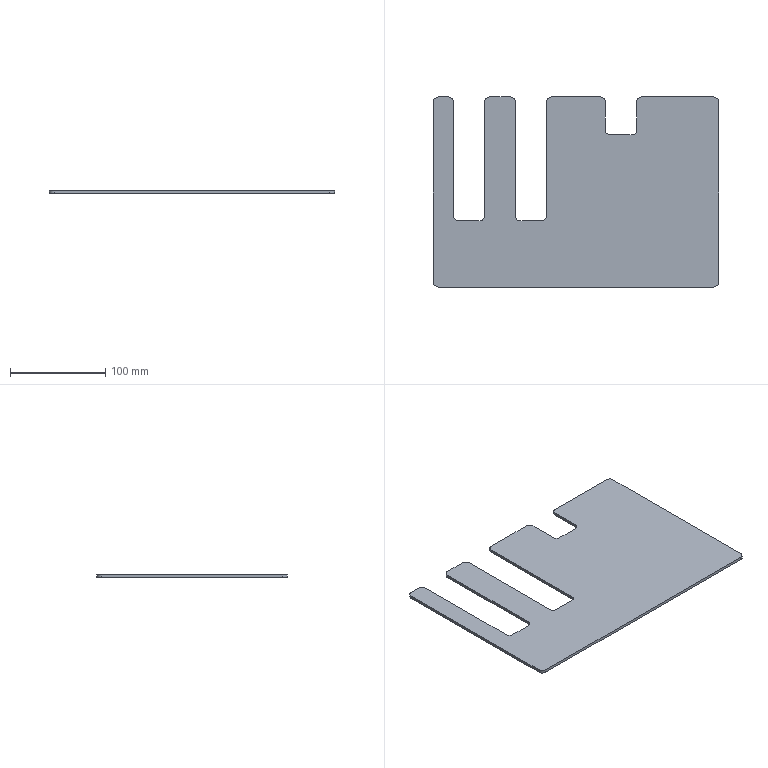Part | STEP file | Sheet21 | 1 solid | 34 faces | box 300 x 200 x 3 mm | volume 150236 mm3 | plane 18 | cylinder 16 | commonest cylinder face diameters 10 x16